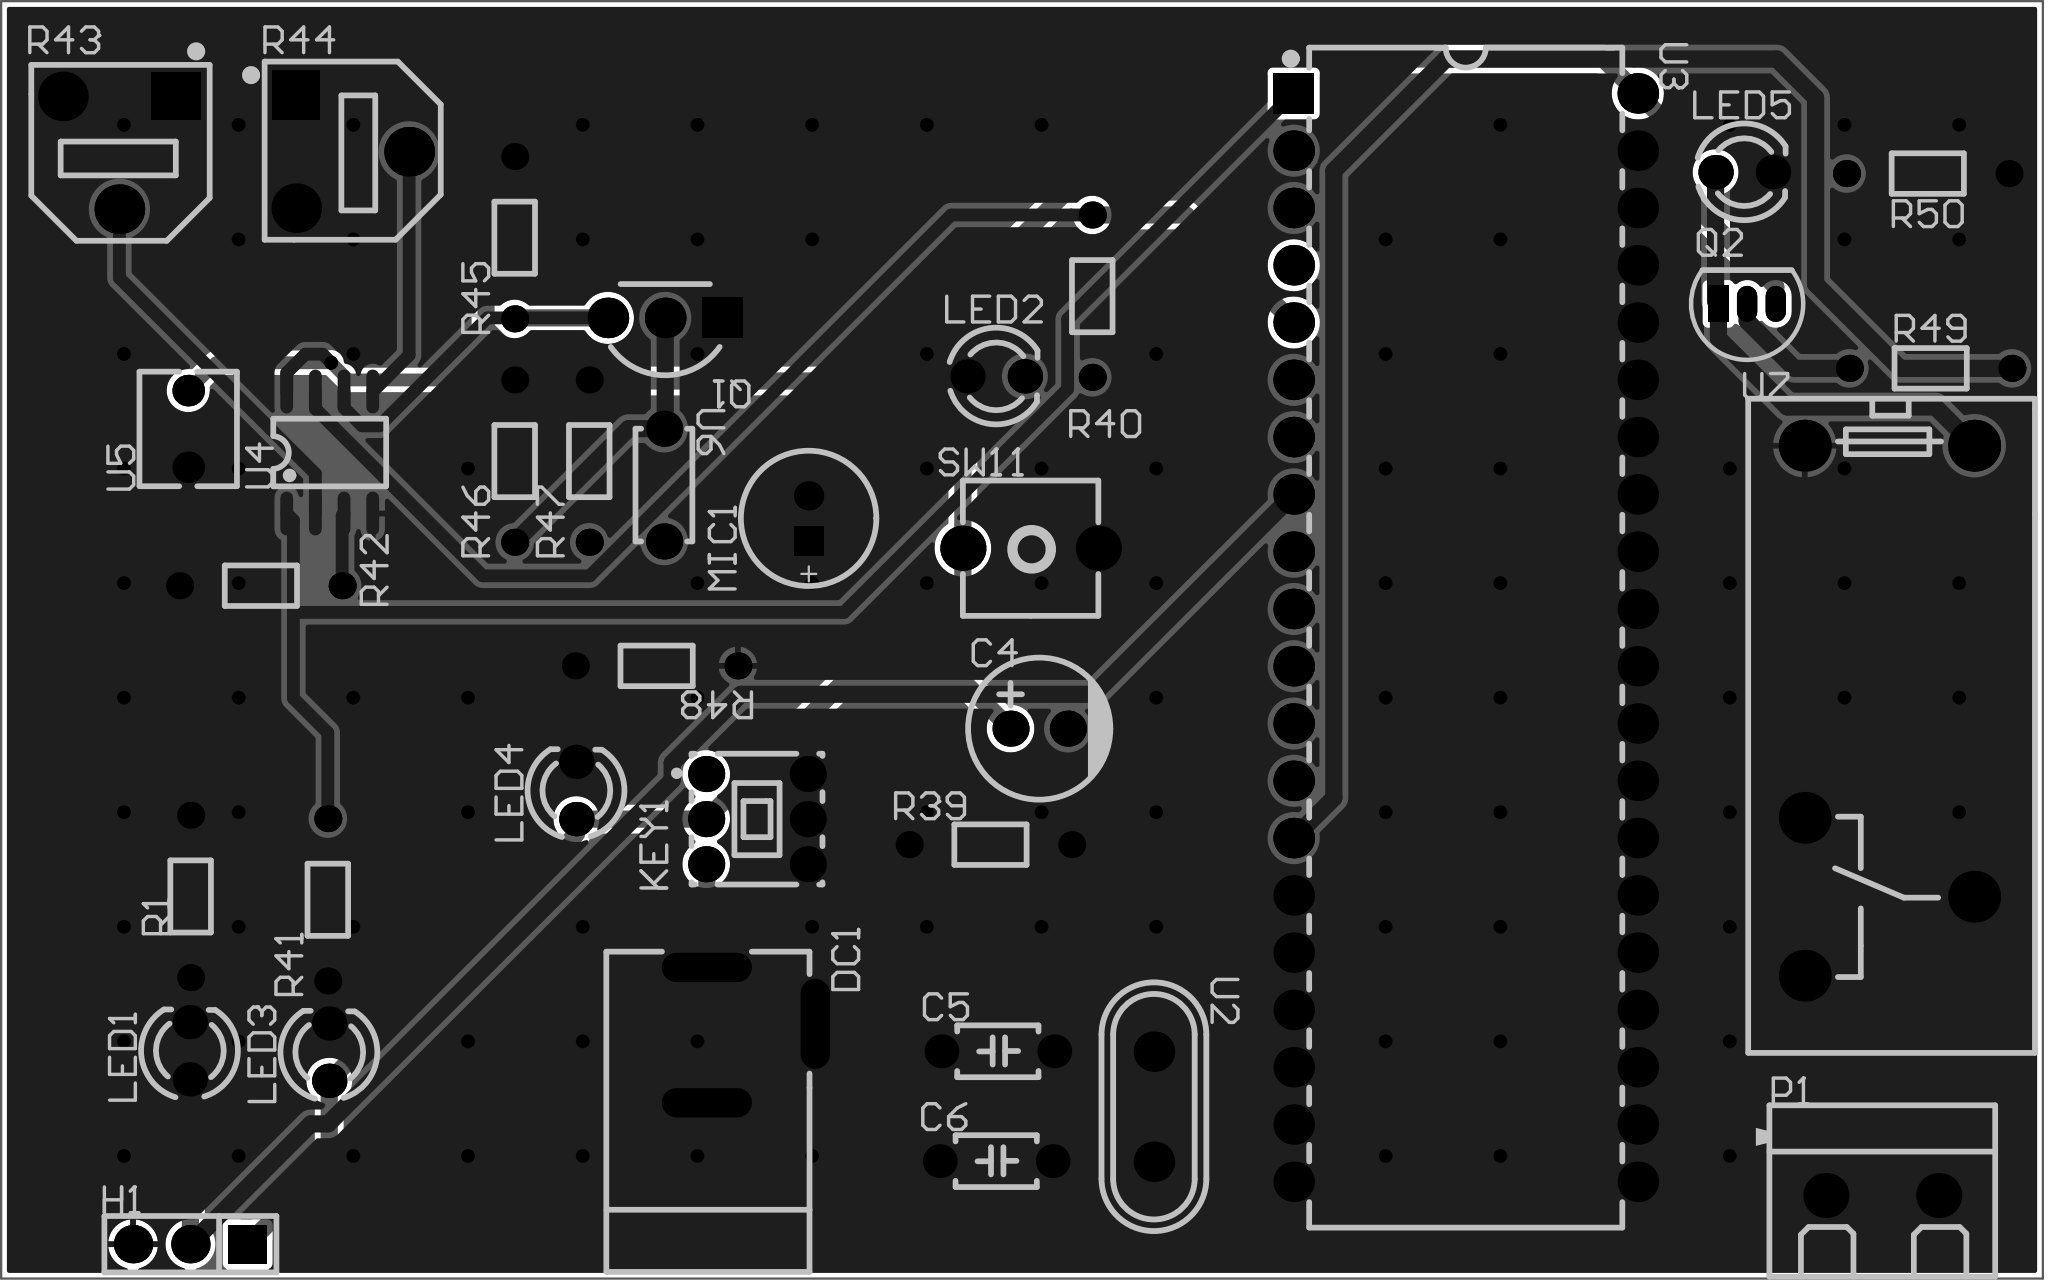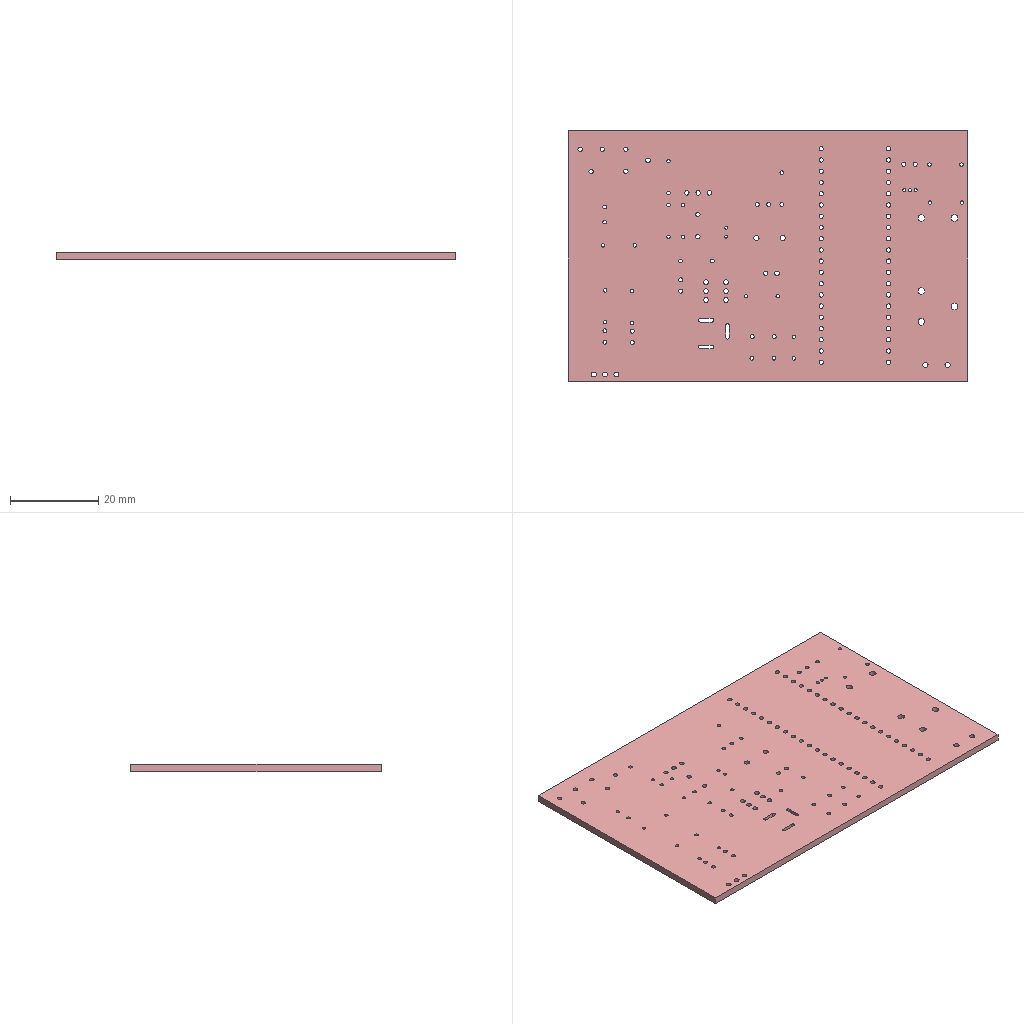Circuit board layout | Altium Designer | box 90.4 x 56.6 x 1.6 mm
Layer stack:
# Altium Designer layer stack of  (unit mm; dielectric type: 0 none, 1 core, 2 prepreg, 3 surface material)
index,name,kind,layer,copper_thickness_mm,dielectric_type,dielectric_thickness_mm,dielectric_material,dielectric_constant
0,Top Paste Mask Layer,other,,,,,,
1,Top Silkscreen Layer,other,,,,,,
2,Top Solder Mask Layer,dielectric,,,3,0.01,,3.3
3,Top Layer,copper,Top Layer,0.035,,,,
4,Dielectric1,dielectric,,,3,1.51,FR4,4.5
5,Bottom Layer,copper,Bottom Layer,0.035,,,,
6,Bottom Solder Mask Layer,dielectric,,,3,0.01,,3.3
7,Bottom Silkscreen Layer,other,,,,,,
8,Bottom Paste Mask Layer,other,,,,,,
# drill layer pairs: low layer,high layer
drill_pair,Top Layer,Bottom Layer
Part placement:
Designator,Comment,Layer,Footprint,Center-X(mm),Center-Y(mm),Rotation
C4,10uF,TopLayer,CAP-TH_BD6.3-P2.50-D1.0-FD,131.699,113.665,0
C5,30pF,TopLayer,CAP-TH_L3.6-W2.3-P5.00-D0.5,129.867,99.359,0
C6,30pF,TopLayer,CAP-TH_L3.6-W2.3-P5.00-D0.5,129.794,94.488,0
DC1,,TopLayer,DC-2.0,119.38,100.076,270
H1,,TopLayer,HDR-TH_3P-P2.54-V-M,94.107,90.805,180
KEY1,Self-locking switch 5.8Z white-grey-white 260G,TopLayer,SW-TH_6P-L5.8-W5.8-P2.00-LS4.5-TR,119.2,109.653,90
LED1,,TopLayer,LED_TH-3mm,94.081,99.383,90
LED2,,TopLayer,LED_TH-3mm,129.794,129.286,0
LED3,,TopLayer,LED_TH-3mm,100.256,99.322,90
LED4,,TopLayer,LED_TH-3mm,111.199,110.923,90
LED5,,TopLayer,LED_TH-3mm,162.923,138.341,0
MIC1,MIC,TopLayer,MIC-TH_BD6.0-P2.00,121.486,122.988,90
P1,KF301-2P terminal block,TopLayer,CONN-TH_XY301V-A-5.0-2P,169.037,92.964,180
Q1,9014,TopLayer,TO-92-3_L4.9-W3.7-P2.54-L,115.136,131.878,180
Q2,9012-H,TopLayer,TO-92-3_L4.9-W3.7-P1.27-R,163.05,132.499,180
R1,2kΩ,TopLayer,Res_1/8W,94.117,106.224,270
R39,10kΩ,TopLayer,Res_1/8W,129.54,108.521,0
R40,2kΩ,TopLayer,Res_1/8W,134.048,132.842,270
R41,2kΩ,TopLayer,Res_1/8W,100.193,106.077,90
R42,2kΩ,TopLayer,Res_1/8W,97.229,120.003,0
R43,10kΩ,TopLayer,RES-ADJ-SMD_RM065-V1,90.962,139.198,180
R44,10kΩ,TopLayer,RES-ADJ-SMD_RM065-V1,101.293,139.244,270
R45,20kΩ,TopLayer,Res_1/8W,108.469,135.434,90
R46,2.2MΩ,TopLayer,Res_1/8W,108.469,125.528,90
R47,10kΩ,TopLayer,Res_1/8W,111.771,125.528,90
R48,2kΩ,TopLayer,Res_1/8W,114.755,116.448,180
R49,2kΩ,TopLayer,Res_1/8W,171.179,129.641,0
R50,2kΩ,TopLayer,Res_1/8W,171.052,138.278,180
SW11,Tact switch, 6*6*5 plastic head, 260G, travel 0.25mm, through-hole, middle 2 pins,TopLayer,KEY-TH_2P-L6.0-W6.0-P5.00,131.318,121.666,0
U2,12MHz,TopLayer,HC-49US_L11.0-W4.6-P4.88,136.779,96.901,270
U3,STC89C516RD+40I-PDIP40,TopLayer,DIP-40_L52.3-W13.9-P2.54-LS15.2-BL,150.589,117.702,270
U4,LM393DR2G,TopLayer,SOIC-8_L5.0-W4.0-P1.27-LS6.0-BL,100.277,125.909,0
U5,光敏电阻-5MM,TopLayer,RES-TH_L4.9-W4.3-P3.4,94.009,126.955,90
U6,100nF,TopLayer,CAP-TH_L5.0-W2.5-P5.00-D1.0,115.088,124.466,270
U7,SSKD6132,TopLayer,RELAY-TH_G2R-1,169.355,114.461,270
Pad and via stacks:
# Altium Designer via and pad stacks of  (unit mm). Each distinct definition once, with the count of objects using it.
# via: kind,start_layer,end_layer,hole_mm,diameter_mm,mode(0 simple;1 top-mid-bottom;2 full stack),diameter_per_layer,count,example_net
# pad: kind,layer,hole_mm,hole_type(0 round;1 square;2 slot),plating,top_size,top_shape(1 round;2 rect;3 octagon;9 rounded rect),mid_size,bottom_size,mode,footprint,size_per_layer,count,example
pad,Multi-Layer,1,0,plated,1.6x1.6,1,1.6x1.6,1.6x1.6,0,CAP-TH_BD6.3-P2.50-D1.0-FD,,2,C4.1
pad,Multi-Layer,0.9,0,plated,1.5x1.5,1,1.5x1.5,1.5x1.5,0,CAP-TH_L3.6-W2.3-P5.00-D0.5,,4,C5.1
pad,Multi-Layer,0.8001,2,plated,4x1.3,1,4x1.3,4x1.3,0,DC-2.0,,3,DC1.2
pad,Multi-Layer,1.1,0,plated,1.7x1.7,2,1.7x1.7,1.7x1.7,0,HDR-TH_3P-P2.54-V-M,,1,H1.1
pad,Multi-Layer,1.1,0,plated,1.7x1.7,1,1.7x1.7,1.7x1.7,0,HDR-TH_3P-P2.54-V-M,,2,H1.2
pad,Multi-Layer,1.1,0,plated,1.6x1.6,1,1.6x1.6,1.6x1.6,0,SW-TH_6P-L5.8-W5.8-P2.00-LS4.5-TR,,6,KEY1.6
pad,Multi-Layer,0.9144,0,plated,1.524x1.524,1,1.524x1.524,1.524x1.524,0,LED_TH-3mm,,10,LED1.1
pad,Multi-Layer,0.7,0,plated,1.3x1.3,2,1.3x1.3,1.3x1.3,0,MIC-TH_BD6.0-P2.00,,1,MIC1.1
pad,Multi-Layer,0.7,0,plated,1.3x1.3,1,1.3x1.3,1.3x1.3,0,MIC-TH_BD6.0-P2.00,,1,MIC1.2
pad,Multi-Layer,1.2,0,plated,2x2,1,2x2,2x2,0,CONN-TH_XY301V-A-5.0-2P,,2,P1.1
pad,Multi-Layer,1,0,plated,1.8x1.8,2,1.8x1.8,1.8x1.8,0,TO-92-3_L4.9-W3.7-P2.54-L,,1,Q1.1
pad,Multi-Layer,1,0,plated,1.8x1.8,1,1.8x1.8,1.8x1.8,0,TO-92-3_L4.9-W3.7-P2.54-L,,2,Q1.2
pad,Multi-Layer,0.7,0,plated,0.9x1.6,1,0.9x1.6,0.9x1.6,0,TO-92-3_L4.9-W3.7-P1.27-R,,2,Q2.3
pad,Multi-Layer,0.7,0,plated,0.9x1.6,2,0.9x1.6,0.9x1.6,0,TO-92-3_L4.9-W3.7-P1.27-R,,1,Q2.1
pad,Multi-Layer,0.8001,0,plated,1.199x1.199,1,1.199x1.199,1.199x1.199,0,Res_1/8W,,22,R1.1
pad,Multi-Layer,1,0,plated,2.2x2.1,2,2.2x2.1,2.2x2.1,0,RES-ADJ-SMD_RM065-V1,,2,R43.1
pad,Multi-Layer,1,0,plated,2.2x2.2,1,2.2x2.2,2.2x2.2,0,RES-ADJ-SMD_RM065-V1,,4,R43.3
pad,Multi-Layer,1.2,0,plated,2x2,1,2x2,2x2,0,KEY-TH_2P-L6.0-W6.0-P5.00,,2,SW11.2
pad,Multi-Layer,0.8,0,plated,1.8x1.8,1,1.8x1.8,1.8x1.8,0,HC-49US_L11.0-W4.6-P4.88,,2,U2.1
pad,Multi-Layer,1,0,plated,1.8x1.8,1,1.8x1.8,1.8x1.8,0,DIP-40_L52.3-W13.9-P2.54-LS15.2-BL,,39,U3.19
pad,Multi-Layer,1,0,plated,1.8x1.8,2,1.8x1.8,1.8x1.8,0,DIP-40_L52.3-W13.9-P2.54-LS15.2-BL,,1,U3.1
pad,Multi-Layer,0.8,0,plated,1.4x1.4,1,1.4x1.4,1.4x1.4,0,RES-TH_L4.9-W4.3-P3.4,,2,U5.1
pad,Multi-Layer,1,0,plated,1.6x1.6,1,1.6x1.6,1.6x1.6,0,CAP-TH_L5.0-W2.5-P5.00-D1.0,,2,U6.1
pad,Multi-Layer,1.5,0,plated,2.3x2.3,1,2.3x2.3,2.3x2.3,0,RELAY-TH_G2R-1,,5,U7.3
pad,Top Layer,0,0,plated,0.5684x1.95,1,0.5684x1.95,0.5684x1.95,0,SOIC-8_L5.0-W4.0-P1.27-LS6.0-BL,,8,U4.1
via,Top Layer,Bottom Layer,0.3048,0.61,0,,101,VCC
Copper pours:
name,layer,net,type(0 solid;1 hatched;2 none)
Top Layer-GND,Top Layer,GND,0
Bottom Layer-GND,Bottom Layer,GND,0
Design rules, without the lines most boards share:
# Altium Designer design rules of  (exported by Altium Designer, unit mm)
# columns: name | kind | enabled | priority | scope1 | scope2 | descriptor | typed fields (field=value)
copperThickness1oz_2 | 2 | enabled | 2 | All | All | Width Constraint (Min=5mil) (Max=100mil) (Preferred=30mil) (All) |
viaSize | 11 | enabled | 1 | All | All | Routing Via (MinHoleWidth=11.811mil) (MaxHoleWidth=248.032mil) (PreferredHoleWidth=12.008mil) (MinWidth=19.685mil) (MaxWidth=393.701mil) (PreferedWidth=24.016mil) (All) | via_min_hole=0.3 via_max_hole=6.3 via_preferred_diameter=0.61 via_preferred_hole=0.305
solderMaskExpansion | 13 | enabled | 2 | All | All | Solder Mask Expansion (Expansion =2.008mil) (All) | expansion=0.051